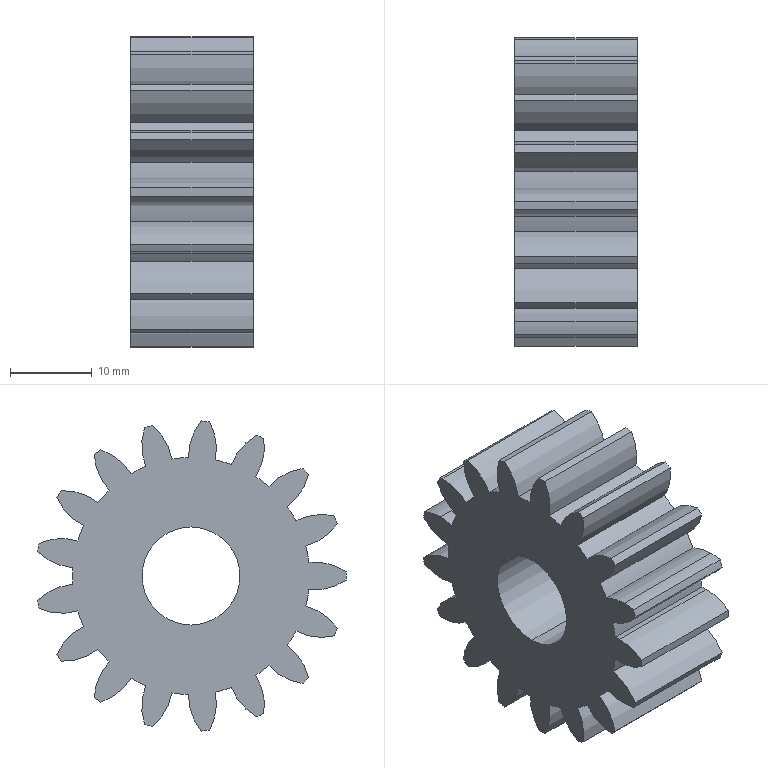Part | SolidWorks | features Boss 3, Cut 3, CirPattern 2, Fillet 2, Revolution 1 | 1 solid | 76 faces | box 15 x 37.761 x 37.916 mm | volume 11362 mm3 | cylinder 74 | plane 2 | commonest cylinder face diameters 13.6 x38 28.998 x17 38 x17 12 x2